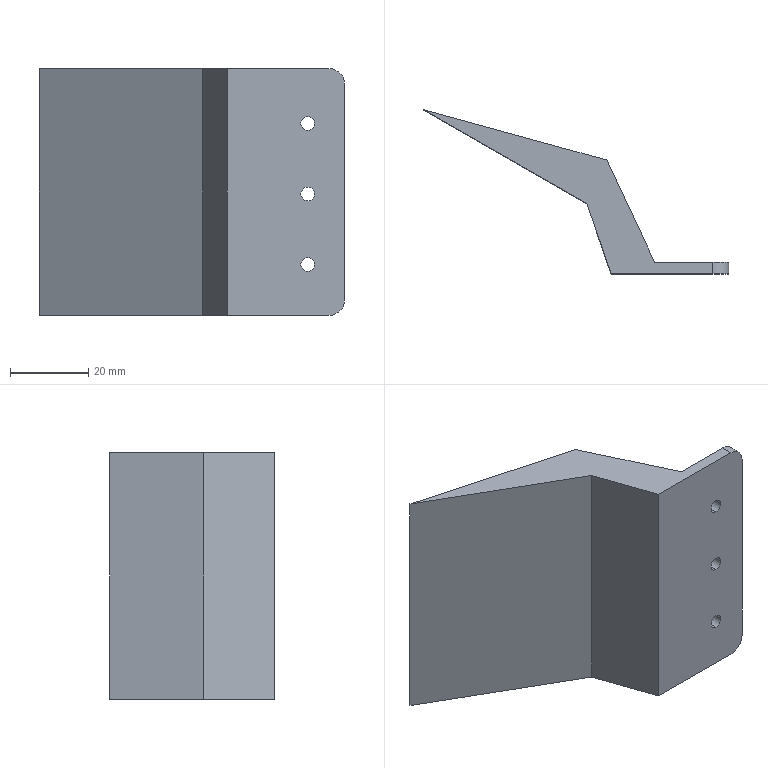Part | SolidWorks | features ICE 2, Extrusion 1, Fillet 1 | 1 solid | 17 faces | box 77.912 x 41.912 x 63 mm | volume 38242 mm3 | plane 9 | cylinder 8 | commonest cylinder face diameters 3.5 x6 8 x2
STEP:
#1=CARTESIAN_POINT('',(20.559,0.,-20.25));
#2=VERTEX_POINT('',#1);
#3=CARTESIAN_POINT('',(20.559,0.,-16.75));
#4=VERTEX_POINT('',#3);
#5=CARTESIAN_POINT('',(20.559,0.,-18.5));
#6=DIRECTION('',(0.,1.,0.));
#7=DIRECTION('',(0.,0.,1.));
#8=AXIS2_PLACEMENT_3D('',#5,#6,#7);
#9=CIRCLE('',#8,1.75);
#10=EDGE_CURVE('',#2,#4,#9,.T.);
#11=ORIENTED_EDGE('',*,*,#10,.F.);
#12=CARTESIAN_POINT('',(20.559,3.,-20.25));
#13=VERTEX_POINT('',#12);
#14=CARTESIAN_POINT('',(20.559,-47.,-20.25));
#15=DIRECTION('',(0.,1.,0.));
#16=VECTOR('',#15,1000.);
#17=LINE('',#14,#16);
#18=EDGE_CURVE('',#2,#13,#17,.T.);
#19=ORIENTED_EDGE('',*,*,#18,.T.);
#20=CARTESIAN_POINT('',(20.559,3.,-16.75));
#21=VERTEX_POINT('',#20);
#22=CARTESIAN_POINT('',(20.559,3.,-18.5));
#23=DIRECTION('',(0.,1.,0.));
#24=DIRECTION('',(0.,0.,1.));
#25=AXIS2_PLACEMENT_3D('',#22,#23,#24);
#26=CIRCLE('',#25,1.75);
#27=EDGE_CURVE('',#13,#21,#26,.T.);
#28=ORIENTED_EDGE('',*,*,#27,.T.);
#29=CARTESIAN_POINT('',(20.559,-47.,-16.75));
#30=DIRECTION('',(0.,1.,0.));
#31=VECTOR('',#30,1000.);
#32=LINE('',#29,#31);
#33=EDGE_CURVE('',#4,#21,#32,.T.);
#34=ORIENTED_EDGE('',*,*,#33,.F.);
#35=EDGE_LOOP('',(#11,#19,#28,#34));
#36=FACE_OUTER_BOUND('',#35,.T.);
#37=CARTESIAN_POINT('',(20.559,-47.,-18.5));
#38=DIRECTION('',(0.,1.,0.));
#39=DIRECTION('',(0.,0.,1.));
#40=AXIS2_PLACEMENT_3D('',#37,#38,#39);
#41=CYLINDRICAL_SURFACE('',#40,1.75);
#42=ADVANCED_FACE('',(#36),#41,.F.);
#43=CARTESIAN_POINT('',(20.559,0.,-2.25));
#44=VERTEX_POINT('',#43);
#45=CARTESIAN_POINT('',(20.559,0.,1.25));
#46=VERTEX_POINT('',#45);
#47=CARTESIAN_POINT('',(20.559,0.,-0.5));
#48=DIRECTION('',(0.,1.,0.));
#49=DIRECTION('',(0.,0.,1.));
#50=AXIS2_PLACEMENT_3D('',#47,#48,#49);
#51=CIRCLE('',#50,1.75);
#52=EDGE_CURVE('',#44,#46,#51,.T.);
#53=ORIENTED_EDGE('',*,*,#52,.F.);
#54=CARTESIAN_POINT('',(20.559,3.,-2.25));
#55=VERTEX_POINT('',#54);
#56=CARTESIAN_POINT('',(20.559,-47.,-2.25));
#57=DIRECTION('',(0.,1.,0.));
#58=VECTOR('',#57,1000.);
#59=LINE('',#56,#58);
#60=EDGE_CURVE('',#44,#55,#59,.T.);
#61=ORIENTED_EDGE('',*,*,#60,.T.);
#62=CARTESIAN_POINT('',(20.559,3.,1.25));
#63=VERTEX_POINT('',#62);
#64=CARTESIAN_POINT('',(20.559,3.,-0.5));
#65=DIRECTION('',(0.,1.,0.));
#66=DIRECTION('',(0.,0.,1.));
#67=AXIS2_PLACEMENT_3D('',#64,#65,#66);
#68=CIRCLE('',#67,1.75);
#69=EDGE_CURVE('',#55,#63,#68,.T.);
#70=ORIENTED_EDGE('',*,*,#69,.T.);
#71=CARTESIAN_POINT('',(20.559,-47.,1.25));
#72=DIRECTION('',(0.,1.,0.));
#73=VECTOR('',#72,1000.);
#74=LINE('',#71,#73);
#75=EDGE_CURVE('',#46,#63,#74,.T.);
#76=ORIENTED_EDGE('',*,*,#75,.F.);
#77=EDGE_LOOP('',(#53,#61,#70,#76));
#78=FACE_OUTER_BOUND('',#77,.T.);
#79=CARTESIAN_POINT('',(20.559,-47.,-0.5));
#80=DIRECTION('',(0.,1.,0.));
#81=DIRECTION('',(0.,0.,1.));
#82=AXIS2_PLACEMENT_3D('',#79,#80,#81);
#83=CYLINDRICAL_SURFACE('',#82,1.75);
#84=ADVANCED_FACE('',(#78),#83,.F.);
#85=CARTESIAN_POINT('',(20.559,0.,15.75));
#86=VERTEX_POINT('',#85);
#87=CARTESIAN_POINT('',(20.559,0.,19.25));
#88=VERTEX_POINT('',#87);
#89=CARTESIAN_POINT('',(20.559,0.,17.5));
#90=DIRECTION('',(0.,1.,0.));
#91=DIRECTION('',(0.,0.,1.));
#92=AXIS2_PLACEMENT_3D('',#89,#90,#91);
#93=CIRCLE('',#92,1.75);
#94=EDGE_CURVE('',#86,#88,#93,.T.);
#95=ORIENTED_EDGE('',*,*,#94,.F.);
#96=CARTESIAN_POINT('',(20.559,3.,15.75));
#97=VERTEX_POINT('',#96);
#98=CARTESIAN_POINT('',(20.559,-47.,15.75));
#99=DIRECTION('',(0.,1.,0.));
#100=VECTOR('',#99,1000.);
#101=LINE('',#98,#100);
#102=EDGE_CURVE('',#86,#97,#101,.T.);
#103=ORIENTED_EDGE('',*,*,#102,.T.);
#104=CARTESIAN_POINT('',(20.559,3.,19.25));
#105=VERTEX_POINT('',#104);
#106=CARTESIAN_POINT('',(20.559,3.,17.5));
#107=DIRECTION('',(0.,1.,0.));
#108=DIRECTION('',(0.,0.,1.));
#109=AXIS2_PLACEMENT_3D('',#106,#107,#108);
#110=CIRCLE('',#109,1.75);
#111=EDGE_CURVE('',#97,#105,#110,.T.);
#112=ORIENTED_EDGE('',*,*,#111,.T.);
#113=CARTESIAN_POINT('',(20.559,-47.,19.25));
#114=DIRECTION('',(0.,1.,0.));
#115=VECTOR('',#114,1000.);
#116=LINE('',#113,#115);
#117=EDGE_CURVE('',#88,#105,#116,.T.);
#118=ORIENTED_EDGE('',*,*,#117,.F.);
#119=EDGE_LOOP('',(#95,#103,#112,#118));
#120=FACE_OUTER_BOUND('',#119,.T.);
#121=CARTESIAN_POINT('',(20.559,-47.,17.5));
#122=DIRECTION('',(0.,1.,0.));
#123=DIRECTION('',(0.,0.,1.));
#124=AXIS2_PLACEMENT_3D('',#121,#122,#123);
#125=CYLINDRICAL_SURFACE('',#124,1.75);
#126=ADVANCED_FACE('',(#120),#125,.F.);
#127=CARTESIAN_POINT('',(20.559,0.,-18.5));
#128=DIRECTION('',(0.,1.,0.));
#129=DIRECTION('',(0.,0.,1.));
#130=AXIS2_PLACEMENT_3D('',#127,#128,#129);
#131=CIRCLE('',#130,1.75);
#132=EDGE_CURVE('',#4,#2,#131,.T.);
#133=ORIENTED_EDGE('',*,*,#132,.T.);
#134=ORIENTED_EDGE('',*,*,#10,.T.);
#135=EDGE_LOOP('',(#133,#134));
#136=FACE_BOUND('',#135,.T.);
#137=CARTESIAN_POINT('',(20.559,0.,-0.5));
#138=DIRECTION('',(0.,1.,0.));
#139=DIRECTION('',(0.,0.,1.));
#140=AXIS2_PLACEMENT_3D('',#137,#138,#139);
#141=CIRCLE('',#140,1.75);
#142=EDGE_CURVE('',#46,#44,#141,.T.);
#143=ORIENTED_EDGE('',*,*,#142,.T.);
#144=ORIENTED_EDGE('',*,*,#52,.T.);
#145=EDGE_LOOP('',(#143,#144));
#146=FACE_BOUND('',#145,.T.);
#147=CARTESIAN_POINT('',(20.559,0.,17.5));
#148=DIRECTION('',(0.,1.,0.));
#149=DIRECTION('',(0.,0.,1.));
#150=AXIS2_PLACEMENT_3D('',#147,#148,#149);
#151=CIRCLE('',#150,1.75);
#152=EDGE_CURVE('',#88,#86,#151,.T.);
#153=ORIENTED_EDGE('',*,*,#152,.T.);
#154=ORIENTED_EDGE('',*,*,#94,.T.);
#155=EDGE_LOOP('',(#153,#154));
#156=FACE_BOUND('',#155,.T.);
#157=CARTESIAN_POINT('',(30.,0.,-27.5));
#158=VERTEX_POINT('',#157);
#159=CARTESIAN_POINT('',(30.,0.,27.5));
#160=VERTEX_POINT('',#159);
#161=CARTESIAN_POINT('',(30.,0.,-61.65));
#162=DIRECTION('',(0.,0.,1.));
#163=VECTOR('',#162,1000.);
#164=LINE('',#161,#163);
#165=EDGE_CURVE('',#158,#160,#164,.T.);
#166=ORIENTED_EDGE('',*,*,#165,.T.);
#167=CARTESIAN_POINT('',(26.,0.,31.5));
#168=VERTEX_POINT('',#167);
#169=CARTESIAN_POINT('',(26.,0.,27.5));
#170=DIRECTION('',(0.,-1.,0.));
#171=DIRECTION('',(0.,0.,1.));
#172=AXIS2_PLACEMENT_3D('',#169,#170,#171);
#173=CIRCLE('',#172,4.);
#174=EDGE_CURVE('',#160,#168,#173,.T.);
#175=ORIENTED_EDGE('',*,*,#174,.T.);
#176=CARTESIAN_POINT('',(0.,0.,31.5));
#177=VERTEX_POINT('',#176);
#178=CARTESIAN_POINT('',(12.518,0.,31.5));
#179=DIRECTION('',(1.,0.,0.));
#180=VECTOR('',#179,1000.);
#181=LINE('',#178,#180);
#182=EDGE_CURVE('',#177,#168,#181,.T.);
#183=ORIENTED_EDGE('',*,*,#182,.F.);
#184=CARTESIAN_POINT('',(0.,0.,-31.5));
#185=VERTEX_POINT('',#184);
#186=CARTESIAN_POINT('',(0.,0.,31.5));
#187=DIRECTION('',(0.,0.,-1.));
#188=VECTOR('',#187,1000.);
#189=LINE('',#186,#188);
#190=EDGE_CURVE('',#177,#185,#189,.T.);
#191=ORIENTED_EDGE('',*,*,#190,.T.);
#192=CARTESIAN_POINT('',(26.,0.,-31.5));
#193=VERTEX_POINT('',#192);
#194=CARTESIAN_POINT('',(12.518,0.,-31.5));
#195=DIRECTION('',(1.,0.,0.));
#196=VECTOR('',#195,1000.);
#197=LINE('',#194,#196);
#198=EDGE_CURVE('',#185,#193,#197,.T.);
#199=ORIENTED_EDGE('',*,*,#198,.T.);
#200=CARTESIAN_POINT('',(26.,0.,-27.5));
#201=DIRECTION('',(0.,-1.,0.));
#202=DIRECTION('',(0.,0.,1.));
#203=AXIS2_PLACEMENT_3D('',#200,#201,#202);
#204=CIRCLE('',#203,4.);
#205=EDGE_CURVE('',#193,#158,#204,.T.);
#206=ORIENTED_EDGE('',*,*,#205,.T.);
#207=EDGE_LOOP('',(#166,#175,#183,#191,#199,#206));
#208=FACE_OUTER_BOUND('',#207,.T.);
#209=CARTESIAN_POINT('',(12.518,0.,31.5));
#210=DIRECTION('',(0.,1.,0.));
#211=DIRECTION('',(0.,0.,1.));
#212=AXIS2_PLACEMENT_3D('',#209,#210,#211);
#213=PLANE('',#212);
#214=ADVANCED_FACE('',(#136,#146,#156,#208),#213,.F.);
#215=CARTESIAN_POINT('',(11.119,3.,31.5));
#216=VERTEX_POINT('',#215);
#217=CARTESIAN_POINT('',(-1.017,29.025,31.5));
#218=VERTEX_POINT('',#217);
#219=CARTESIAN_POINT('',(-1.017,29.025,31.5));
#220=DIRECTION('',(-0.4226,0.9063,0.));
#221=VECTOR('',#220,1000.);
#222=LINE('',#219,#221);
#223=EDGE_CURVE('',#216,#218,#222,.T.);
#224=ORIENTED_EDGE('',*,*,#223,.F.);
#225=CARTESIAN_POINT('',(11.119,3.,-31.5));
#226=VERTEX_POINT('',#225);
#227=CARTESIAN_POINT('',(11.119,3.,31.5));
#228=DIRECTION('',(0.,0.,-1.));
#229=VECTOR('',#228,1000.);
#230=LINE('',#227,#229);
#231=EDGE_CURVE('',#216,#226,#230,.T.);
#232=ORIENTED_EDGE('',*,*,#231,.T.);
#233=CARTESIAN_POINT('',(-1.017,29.025,-31.5));
#234=VERTEX_POINT('',#233);
#235=CARTESIAN_POINT('',(-1.017,29.025,-31.5));
#236=DIRECTION('',(-0.4226,0.9063,0.));
#237=VECTOR('',#236,1000.);
#238=LINE('',#235,#237);
#239=EDGE_CURVE('',#226,#234,#238,.T.);
#240=ORIENTED_EDGE('',*,*,#239,.T.);
#241=CARTESIAN_POINT('',(-1.017,29.025,31.5));
#242=DIRECTION('',(0.,0.,-1.));
#243=VECTOR('',#242,1000.);
#244=LINE('',#241,#243);
#245=EDGE_CURVE('',#218,#234,#244,.T.);
#246=ORIENTED_EDGE('',*,*,#245,.F.);
#247=EDGE_LOOP('',(#224,#232,#240,#246));
#248=FACE_OUTER_BOUND('',#247,.T.);
#249=CARTESIAN_POINT('',(-1.017,29.025,31.5));
#250=DIRECTION('',(-0.9063,-0.4226,0.));
#251=DIRECTION('',(0.4226,-0.9063,0.));
#252=AXIS2_PLACEMENT_3D('',#249,#250,#251);
#253=PLANE('',#252);
#254=ADVANCED_FACE('',(#248),#253,.F.);
#255=CARTESIAN_POINT('',(-47.912,41.912,-31.5));
#256=VERTEX_POINT('',#255);
#257=CARTESIAN_POINT('',(-47.912,41.912,-31.5));
#258=DIRECTION('',(-0.9643,0.265,0.));
#259=VECTOR('',#258,1000.);
#260=LINE('',#257,#259);
#261=EDGE_CURVE('',#234,#256,#260,.T.);
#262=ORIENTED_EDGE('',*,*,#261,.T.);
#263=CARTESIAN_POINT('',(-47.912,41.912,31.5));
#264=VERTEX_POINT('',#263);
#265=CARTESIAN_POINT('',(-47.912,41.912,31.5));
#266=DIRECTION('',(0.,0.,-1.));
#267=VECTOR('',#266,1000.);
#268=LINE('',#265,#267);
#269=EDGE_CURVE('',#264,#256,#268,.T.);
#270=ORIENTED_EDGE('',*,*,#269,.F.);
#271=CARTESIAN_POINT('',(-47.912,41.912,31.5));
#272=DIRECTION('',(-0.9643,0.265,0.));
#273=VECTOR('',#272,1000.);
#274=LINE('',#271,#273);
#275=EDGE_CURVE('',#218,#264,#274,.T.);
#276=ORIENTED_EDGE('',*,*,#275,.F.);
#277=ORIENTED_EDGE('',*,*,#245,.T.);
#278=EDGE_LOOP('',(#262,#270,#276,#277));
#279=FACE_OUTER_BOUND('',#278,.T.);
#280=CARTESIAN_POINT('',(-47.912,41.912,31.5));
#281=DIRECTION('',(-0.265,-0.9643,0.));
#282=DIRECTION('',(0.9643,-0.265,0.));
#283=AXIS2_PLACEMENT_3D('',#280,#281,#282);
#284=PLANE('',#283);
#285=ADVANCED_FACE('',(#279),#284,.F.);
#286=CARTESIAN_POINT('',(-6.19,18.,-31.5));
#287=VERTEX_POINT('',#286);
#288=CARTESIAN_POINT('',(-6.19,18.,-31.5));
#289=DIRECTION('',(0.8676,-0.4972,0.));
#290=VECTOR('',#289,1000.);
#291=LINE('',#288,#290);
#292=EDGE_CURVE('',#256,#287,#291,.T.);
#293=ORIENTED_EDGE('',*,*,#292,.T.);
#294=CARTESIAN_POINT('',(-6.19,18.,31.5));
#295=VERTEX_POINT('',#294);
#296=CARTESIAN_POINT('',(-6.19,18.,31.5));
#297=DIRECTION('',(0.,0.,-1.));
#298=VECTOR('',#297,1000.);
#299=LINE('',#296,#298);
#300=EDGE_CURVE('',#295,#287,#299,.T.);
#301=ORIENTED_EDGE('',*,*,#300,.F.);
#302=CARTESIAN_POINT('',(-6.19,18.,31.5));
#303=DIRECTION('',(0.8676,-0.4972,0.));
#304=VECTOR('',#303,1000.);
#305=LINE('',#302,#304);
#306=EDGE_CURVE('',#264,#295,#305,.T.);
#307=ORIENTED_EDGE('',*,*,#306,.F.);
#308=ORIENTED_EDGE('',*,*,#269,.T.);
#309=EDGE_LOOP('',(#293,#301,#307,#308));
#310=FACE_OUTER_BOUND('',#309,.T.);
#311=CARTESIAN_POINT('',(-6.19,18.,31.5));
#312=DIRECTION('',(0.4972,0.8676,0.));
#313=DIRECTION('',(-0.8676,0.4972,0.));
#314=AXIS2_PLACEMENT_3D('',#311,#312,#313);
#315=PLANE('',#314);
#316=ADVANCED_FACE('',(#310),#315,.F.);
#317=CARTESIAN_POINT('',(0.,0.,-31.5));
#318=DIRECTION('',(0.3252,-0.9457,0.));
#319=VECTOR('',#318,1000.);
#320=LINE('',#317,#319);
#321=EDGE_CURVE('',#287,#185,#320,.T.);
#322=ORIENTED_EDGE('',*,*,#321,.T.);
#323=ORIENTED_EDGE('',*,*,#190,.F.);
#324=CARTESIAN_POINT('',(0.,0.,31.5));
#325=DIRECTION('',(0.3252,-0.9457,0.));
#326=VECTOR('',#325,1000.);
#327=LINE('',#324,#326);
#328=EDGE_CURVE('',#295,#177,#327,.T.);
#329=ORIENTED_EDGE('',*,*,#328,.F.);
#330=ORIENTED_EDGE('',*,*,#300,.T.);
#331=EDGE_LOOP('',(#322,#323,#329,#330));
#332=FACE_OUTER_BOUND('',#331,.T.);
#333=CARTESIAN_POINT('',(0.,0.,31.5));
#334=DIRECTION('',(0.9457,0.3252,0.));
#335=DIRECTION('',(-0.3252,0.9457,0.));
#336=AXIS2_PLACEMENT_3D('',#333,#334,#335);
#337=PLANE('',#336);
#338=ADVANCED_FACE('',(#332),#337,.F.);
#339=ORIENTED_EDGE('',*,*,#182,.T.);
#340=CARTESIAN_POINT('',(26.,3.,31.5));
#341=VERTEX_POINT('',#340);
#342=CARTESIAN_POINT('',(26.,3.,31.5));
#343=DIRECTION('',(0.,1.,0.));
#344=VECTOR('',#343,1000.);
#345=LINE('',#342,#344);
#346=EDGE_CURVE('',#168,#341,#345,.T.);
#347=ORIENTED_EDGE('',*,*,#346,.T.);
#348=CARTESIAN_POINT('',(0.,3.,31.5));
#349=DIRECTION('',(-1.,0.,0.));
#350=VECTOR('',#349,1000.);
#351=LINE('',#348,#350);
#352=EDGE_CURVE('',#341,#216,#351,.T.);
#353=ORIENTED_EDGE('',*,*,#352,.T.);
#354=ORIENTED_EDGE('',*,*,#223,.T.);
#355=ORIENTED_EDGE('',*,*,#275,.T.);
#356=ORIENTED_EDGE('',*,*,#306,.T.);
#357=ORIENTED_EDGE('',*,*,#328,.T.);
#358=EDGE_LOOP('',(#339,#347,#353,#354,#355,#356,#357));
#359=FACE_OUTER_BOUND('',#358,.T.);
#360=CARTESIAN_POINT('',(0.,0.,31.5));
#361=DIRECTION('',(0.,0.,-1.));
#362=DIRECTION('',(-1.,0.,0.));
#363=AXIS2_PLACEMENT_3D('',#360,#361,#362);
#364=PLANE('',#363);
#365=ADVANCED_FACE('',(#359),#364,.F.);
#366=CARTESIAN_POINT('',(26.,3.,-31.5));
#367=VERTEX_POINT('',#366);
#368=CARTESIAN_POINT('',(0.,3.,-31.5));
#369=DIRECTION('',(-1.,0.,0.));
#370=VECTOR('',#369,1000.);
#371=LINE('',#368,#370);
#372=EDGE_CURVE('',#367,#226,#371,.T.);
#373=ORIENTED_EDGE('',*,*,#372,.F.);
#374=CARTESIAN_POINT('',(26.,0.,-31.5));
#375=DIRECTION('',(0.,-1.,0.));
#376=VECTOR('',#375,1000.);
#377=LINE('',#374,#376);
#378=EDGE_CURVE('',#367,#193,#377,.T.);
#379=ORIENTED_EDGE('',*,*,#378,.T.);
#380=ORIENTED_EDGE('',*,*,#198,.F.);
#381=ORIENTED_EDGE('',*,*,#321,.F.);
#382=ORIENTED_EDGE('',*,*,#292,.F.);
#383=ORIENTED_EDGE('',*,*,#261,.F.);
#384=ORIENTED_EDGE('',*,*,#239,.F.);
#385=EDGE_LOOP('',(#373,#379,#380,#381,#382,#383,#384));
#386=FACE_OUTER_BOUND('',#385,.T.);
#387=CARTESIAN_POINT('',(0.,0.,-31.5));
#388=DIRECTION('',(0.,0.,-1.));
#389=DIRECTION('',(-1.,0.,0.));
#390=AXIS2_PLACEMENT_3D('',#387,#388,#389);
#391=PLANE('',#390);
#392=ADVANCED_FACE('',(#386),#391,.T.);
#393=CARTESIAN_POINT('',(20.559,3.,-18.5));
#394=DIRECTION('',(0.,1.,0.));
#395=DIRECTION('',(0.,0.,1.));
#396=AXIS2_PLACEMENT_3D('',#393,#394,#395);
#397=CIRCLE('',#396,1.75);
#398=EDGE_CURVE('',#21,#13,#397,.T.);
#399=ORIENTED_EDGE('',*,*,#398,.F.);
#400=ORIENTED_EDGE('',*,*,#27,.F.);
#401=EDGE_LOOP('',(#399,#400));
#402=FACE_BOUND('',#401,.T.);
#403=CARTESIAN_POINT('',(20.559,3.,-0.5));
#404=DIRECTION('',(0.,1.,0.));
#405=DIRECTION('',(0.,0.,1.));
#406=AXIS2_PLACEMENT_3D('',#403,#404,#405);
#407=CIRCLE('',#406,1.75);
#408=EDGE_CURVE('',#63,#55,#407,.T.);
#409=ORIENTED_EDGE('',*,*,#408,.F.);
#410=ORIENTED_EDGE('',*,*,#69,.F.);
#411=EDGE_LOOP('',(#409,#410));
#412=FACE_BOUND('',#411,.T.);
#413=CARTESIAN_POINT('',(20.559,3.,17.5));
#414=DIRECTION('',(0.,1.,0.));
#415=DIRECTION('',(0.,0.,1.));
#416=AXIS2_PLACEMENT_3D('',#413,#414,#415);
#417=CIRCLE('',#416,1.75);
#418=EDGE_CURVE('',#105,#97,#417,.T.);
#419=ORIENTED_EDGE('',*,*,#418,.F.);
#420=ORIENTED_EDGE('',*,*,#111,.F.);
#421=EDGE_LOOP('',(#419,#420));
#422=FACE_BOUND('',#421,.T.);
#423=ORIENTED_EDGE('',*,*,#352,.F.);
#424=CARTESIAN_POINT('',(30.,3.,27.5));
#425=VERTEX_POINT('',#424);
#426=CARTESIAN_POINT('',(26.,3.,27.5));
#427=DIRECTION('',(0.,1.,0.));
#428=DIRECTION('',(0.,0.,1.));
#429=AXIS2_PLACEMENT_3D('',#426,#427,#428);
#430=CIRCLE('',#429,4.);
#431=EDGE_CURVE('',#341,#425,#430,.T.);
#432=ORIENTED_EDGE('',*,*,#431,.T.);
#433=CARTESIAN_POINT('',(30.,3.,-27.5));
#434=VERTEX_POINT('',#433);
#435=CARTESIAN_POINT('',(30.,3.,-61.65));
#436=DIRECTION('',(0.,0.,1.));
#437=VECTOR('',#436,1000.);
#438=LINE('',#435,#437);
#439=EDGE_CURVE('',#434,#425,#438,.T.);
#440=ORIENTED_EDGE('',*,*,#439,.F.);
#441=CARTESIAN_POINT('',(26.,3.,-27.5));
#442=DIRECTION('',(0.,1.,0.));
#443=DIRECTION('',(0.,0.,1.));
#444=AXIS2_PLACEMENT_3D('',#441,#442,#443);
#445=CIRCLE('',#444,4.);
#446=EDGE_CURVE('',#434,#367,#445,.T.);
#447=ORIENTED_EDGE('',*,*,#446,.T.);
#448=ORIENTED_EDGE('',*,*,#372,.T.);
#449=ORIENTED_EDGE('',*,*,#231,.F.);
#450=EDGE_LOOP('',(#423,#432,#440,#447,#448,#449));
#451=FACE_OUTER_BOUND('',#450,.T.);
#452=CARTESIAN_POINT('',(0.,3.,-61.65));
#453=DIRECTION('',(0.,1.,0.));
#454=DIRECTION('',(0.,0.,1.));
#455=AXIS2_PLACEMENT_3D('',#452,#453,#454);
#456=PLANE('',#455);
#457=ADVANCED_FACE('',(#402,#412,#422,#451),#456,.T.);
#458=ORIENTED_EDGE('',*,*,#439,.T.);
#459=CARTESIAN_POINT('',(30.,0.,27.5));
#460=DIRECTION('',(0.,-1.,0.));
#461=VECTOR('',#460,1000.);
#462=LINE('',#459,#461);
#463=EDGE_CURVE('',#425,#160,#462,.T.);
#464=ORIENTED_EDGE('',*,*,#463,.T.);
#465=ORIENTED_EDGE('',*,*,#165,.F.);
#466=CARTESIAN_POINT('',(30.,0.,-27.5));
#467=DIRECTION('',(0.,1.,0.));
#468=VECTOR('',#467,1000.);
#469=LINE('',#466,#468);
#470=EDGE_CURVE('',#158,#434,#469,.T.);
#471=ORIENTED_EDGE('',*,*,#470,.T.);
#472=EDGE_LOOP('',(#458,#464,#465,#471));
#473=FACE_OUTER_BOUND('',#472,.T.);
#474=CARTESIAN_POINT('',(30.,0.,-61.65));
#475=DIRECTION('',(1.,0.,0.));
#476=DIRECTION('',(0.,0.,-1.));
#477=AXIS2_PLACEMENT_3D('',#474,#475,#476);
#478=PLANE('',#477);
#479=ADVANCED_FACE('',(#473),#478,.T.);
#480=ORIENTED_EDGE('',*,*,#102,.F.);
#481=ORIENTED_EDGE('',*,*,#152,.F.);
#482=ORIENTED_EDGE('',*,*,#117,.T.);
#483=ORIENTED_EDGE('',*,*,#418,.T.);
#484=EDGE_LOOP('',(#480,#481,#482,#483));
#485=FACE_OUTER_BOUND('',#484,.T.);
#486=CARTESIAN_POINT('',(20.559,-47.,17.5));
#487=DIRECTION('',(0.,1.,0.));
#488=DIRECTION('',(0.,0.,1.));
#489=AXIS2_PLACEMENT_3D('',#486,#487,#488);
#490=CYLINDRICAL_SURFACE('',#489,1.75);
#491=ADVANCED_FACE('',(#485),#490,.F.);
#492=ORIENTED_EDGE('',*,*,#60,.F.);
#493=ORIENTED_EDGE('',*,*,#142,.F.);
#494=ORIENTED_EDGE('',*,*,#75,.T.);
#495=ORIENTED_EDGE('',*,*,#408,.T.);
#496=EDGE_LOOP('',(#492,#493,#494,#495));
#497=FACE_OUTER_BOUND('',#496,.T.);
#498=CARTESIAN_POINT('',(20.559,-47.,-0.5));
#499=DIRECTION('',(0.,1.,0.));
#500=DIRECTION('',(0.,0.,1.));
#501=AXIS2_PLACEMENT_3D('',#498,#499,#500);
#502=CYLINDRICAL_SURFACE('',#501,1.75);
#503=ADVANCED_FACE('',(#497),#502,.F.);
#504=ORIENTED_EDGE('',*,*,#18,.F.);
#505=ORIENTED_EDGE('',*,*,#132,.F.);
#506=ORIENTED_EDGE('',*,*,#33,.T.);
#507=ORIENTED_EDGE('',*,*,#398,.T.);
#508=EDGE_LOOP('',(#504,#505,#506,#507));
#509=FACE_OUTER_BOUND('',#508,.T.);
#510=CARTESIAN_POINT('',(20.559,-47.,-18.5));
#511=DIRECTION('',(0.,1.,0.));
#512=DIRECTION('',(0.,0.,1.));
#513=AXIS2_PLACEMENT_3D('',#510,#511,#512);
#514=CYLINDRICAL_SURFACE('',#513,1.75);
#515=ADVANCED_FACE('',(#509),#514,.F.);
#516=ORIENTED_EDGE('',*,*,#174,.F.);
#517=ORIENTED_EDGE('',*,*,#463,.F.);
#518=ORIENTED_EDGE('',*,*,#431,.F.);
#519=ORIENTED_EDGE('',*,*,#346,.F.);
#520=EDGE_LOOP('',(#516,#517,#518,#519));
#521=FACE_OUTER_BOUND('',#520,.T.);
#522=CARTESIAN_POINT('',(26.,0.,27.5));
#523=DIRECTION('',(0.,-1.,0.));
#524=DIRECTION('',(0.,0.,-1.));
#525=AXIS2_PLACEMENT_3D('',#522,#523,#524);
#526=CYLINDRICAL_SURFACE('',#525,4.);
#527=ADVANCED_FACE('',(#521),#526,.T.);
#528=ORIENTED_EDGE('',*,*,#205,.F.);
#529=ORIENTED_EDGE('',*,*,#378,.F.);
#530=ORIENTED_EDGE('',*,*,#446,.F.);
#531=ORIENTED_EDGE('',*,*,#470,.F.);
#532=EDGE_LOOP('',(#528,#529,#530,#531));
#533=FACE_OUTER_BOUND('',#532,.T.);
#534=CARTESIAN_POINT('',(26.,0.,-27.5));
#535=DIRECTION('',(0.,1.,0.));
#536=DIRECTION('',(0.,0.,1.));
#537=AXIS2_PLACEMENT_3D('',#534,#535,#536);
#538=CYLINDRICAL_SURFACE('',#537,4.);
#539=ADVANCED_FACE('',(#533),#538,.T.);
#540=CLOSED_SHELL('',(#42,#84,#126,#214,#254,#285,#316,#338,#365,#392,#457,#479,#491,#503,#515,#527,#539));
#541=MANIFOLD_SOLID_BREP('',#540);
#542=CARTESIAN_POINT('',(0.,0.,0.));
#543=DIRECTION('',(0.,0.,1.));
#544=DIRECTION('',(1.,0.,0.));
#545=AXIS2_PLACEMENT_3D('',#542,#543,#544);
#546=(LENGTH_UNIT()NAMED_UNIT(*)SI_UNIT(.MILLI.,.METRE.));
#547=UNCERTAINTY_MEASURE_WITH_UNIT(LENGTH_MEASURE(0.00001),#546,'','');
#548=(NAMED_UNIT(*)PLANE_ANGLE_UNIT()SI_UNIT($,.RADIAN.));
#549=(NAMED_UNIT(*)SI_UNIT($,.STERADIAN.)SOLID_ANGLE_UNIT());
#550=(GEOMETRIC_REPRESENTATION_CONTEXT(3)GLOBAL_UNCERTAINTY_ASSIGNED_CONTEXT((#547))GLOBAL_UNIT_ASSIGNED_CONTEXT((#546,#548,#549))REPRESENTATION_CONTEXT('',''));
#551=ADVANCED_BREP_SHAPE_REPRESENTATION('',(#541,#545),#550);